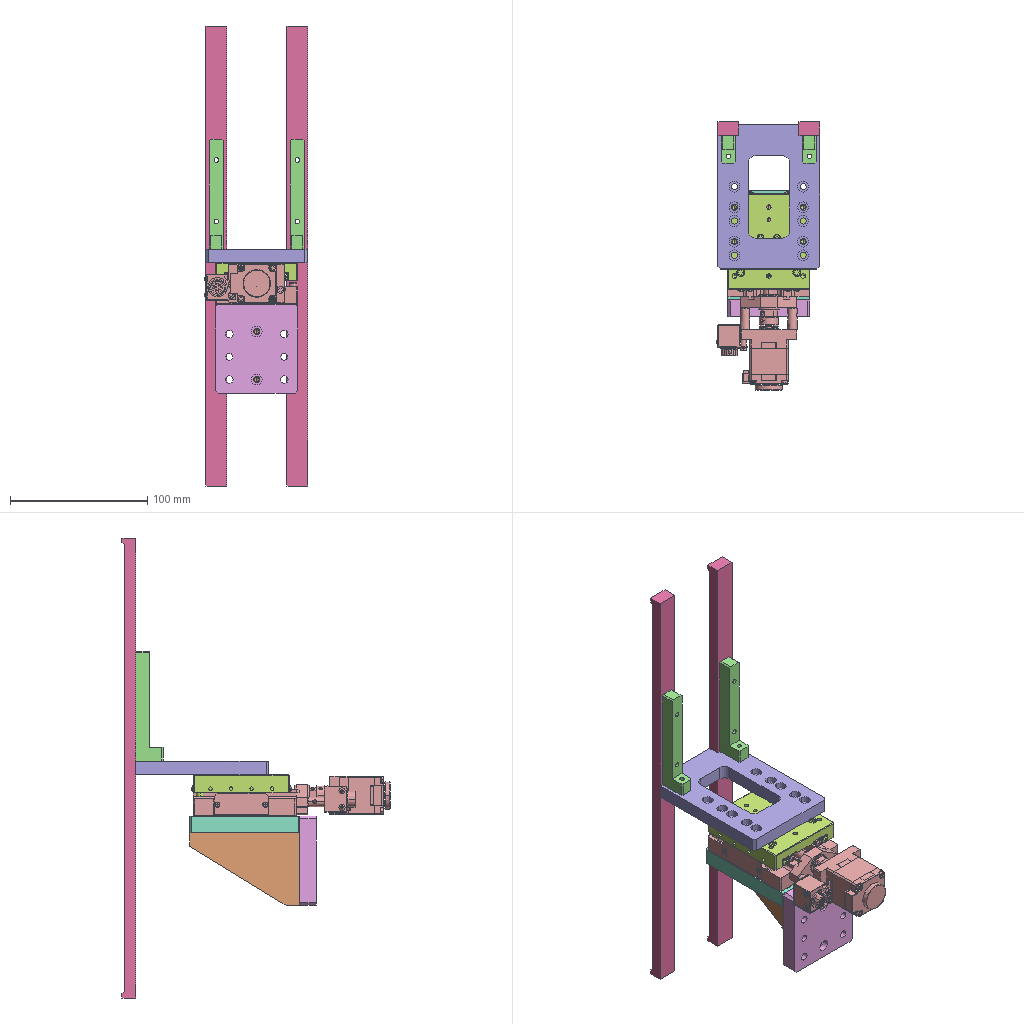Assembly | SolidWorks | 9 different items | 11 placed | box 75 x 195 x 335 mm
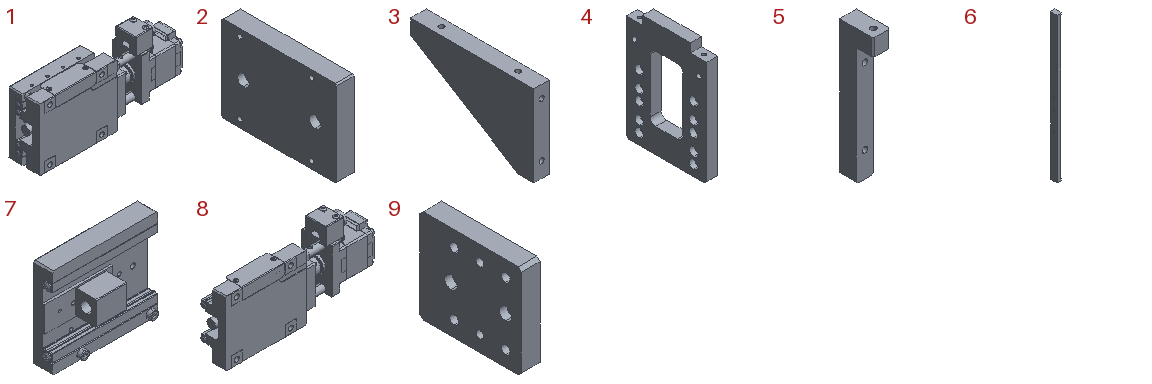Parts list (item | name | quantity | parent item | size | volume | features):
1 | (subassembly) | x1 | - | 144.767 x 30 x 68.134 mm | 145224 mm3 | -
2 | - | x1 | - | 12 x 80 x 60 mm | 56468 mm3 | features HoleWzd 2, Chamfer 1, Extrusion 1
3 | - | x1 | - | 10 x 80 x 53 mm | 26993 mm3 | features HoleWzd 2, Extrusion 1
4 | - | x1 | - | 10 x 74 x 105 mm | 53491 mm3 | features HoleWzd 4, Cut 2, MoveFace 2, Chamfer 1, DelFace 1, Extrusion 1, ICE 1
5 | - | x2 | - | 10 x 20 x 80 mm | 8723 mm3 | features HoleWzd 2, Chamfer 1, Extrusion 1, ICE 1
6 | - | x2 | - | 10 x 15 x 335 mm | 39599 mm3 | features Extrusion 1, HoleWzd 1, ICE 1
7 | - | x1 | in 1 | 72.934 x 22 x 60 mm | 41996 mm3 | features BaseBody 1
8 | - | x1 | in 1 | 144.767 x 29 x 68.134 mm | 103226 mm3 | features BaseBody 23
9 | - | x1 | - | 12 x 65 x 60 mm | 43146 mm3 | features HoleWzd 3, Chamfer 1, Extrusion 1
Mates (type | each side: item.copy, entity, surface, feature):
In the top assembly
Coincident | 2.1 face plane Boss-Extrude1 | 9.1 face plane Boss-Extrude1 | 3 times
Coincident | 3.1 face plane Boss-Extrude1 | 9.1 face plane Boss-Extrude1 | 2 times
Width | 9.1 face plane Boss-Extrude1 | 9.1 face plane Boss-Extrude1 | 3.1 face plane Boss-Extrude1 | 3.1 face plane Boss-Extrude1
Coincident | 2.1 face plane Boss-Extrude1 | 8.1 face plane Input1
Width | 8.1 face plane Input1 | 8.1 face plane Input1 | 2.1 face plane Boss-Extrude1 | 2.1 face plane Boss-Extrude1
Width | 2.1 face plane Boss-Extrude1 | 9.1 face plane Boss-Extrude1 | 8.1 face plane Input1 | 8.1 face plane Input1
Coincident | 4.1 face plane Boss-Extrude1 | 7.1 face plane Input24
Width | 4.1 face plane Boss-Extrude1 | 4.1 face plane Boss-Extrude1 | 7.1 face plane Input24 | 7.1 face plane Input24
Coincident | 4.1 face plane Cut-Extrude2 | 6.1 face plane Boss-Extrude1
Coincident | 6.2 face plane Boss-Extrude1 | 6.1 face plane Boss-Extrude1
Width | 6.1 face plane Boss-Extrude1 | 6.1 face plane Boss-Extrude1 | 4.1 face plane Boss-Extrude1 | 4.1 face plane Boss-Extrude1
Width | 6.2 face plane Boss-Extrude1 | 6.1 face plane Boss-Extrude1 | 4.1 face plane Cut-Extrude2 | 4.1 face plane Cut-Extrude2
Coincident | 4.1 face plane Cut-Extrude2 | 6.2 face plane Boss-Extrude1
Coincident | 4.1 face plane Boss-Extrude1 | 6.2 face plane Boss-Extrude1
Concentric | 6.2 face cylinder CBORE for M4 Hexagon socket head cap screws1 | 5.1 face cylinder M4 Tapped Hole1
Coincident | 4.1 face plane Boss-Extrude1 | 5.1 face plane Boss-Extrude1
Coincident | 6.2 face plane Boss-Extrude1 | 5.1 face plane Boss-Extrude1
Concentric | 6.1 face cylinder CBORE for M4 Hexagon socket head cap screws1 | 5.2 face cylinder M4 Tapped Hole1
Coincident | 6.1 face plane Boss-Extrude1 | 5.2 face plane Boss-Extrude1
Width | 6.1 face plane Boss-Extrude1 | 6.1 face plane Boss-Extrude1 | 5.2 face plane Boss-Extrude1 | 5.2 face plane Boss-Extrude1
Concentric | 7.1 face cylinder Input24 | 4.1 face cylinder CBORE for M4 Hexagon socket head cap screws4
In subassembly 1
Parallel | 8.2 face plane Input1 | 7.2 face plane Input24
Concentric | 8.2 face cylinder Input1 | 7.2 face cylinder Input24
LimitDistanceDim | 7.2 face plane Input24 | 8.2 face plane Input1